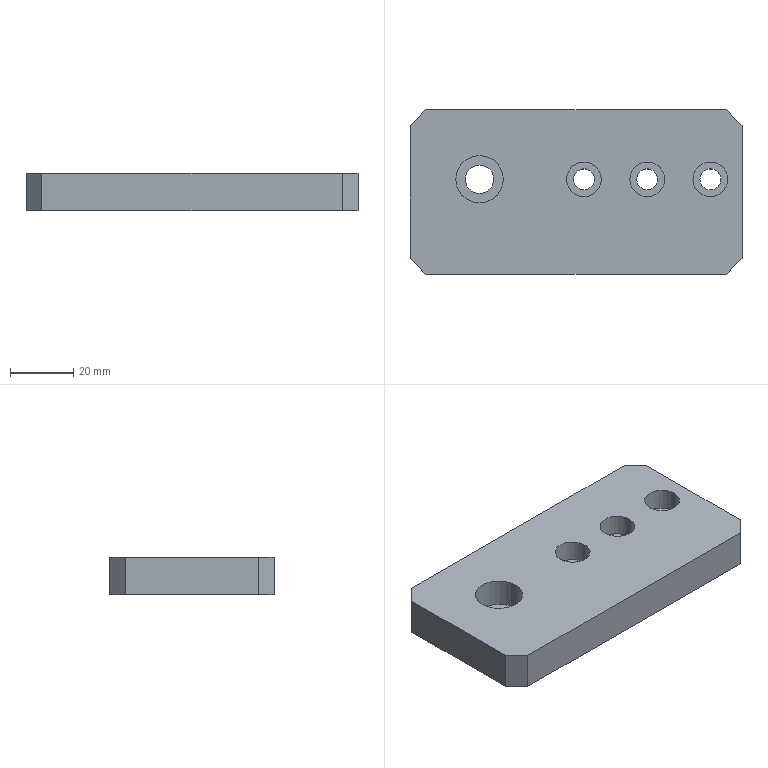Part | STEP file | Driven wheel fixing plate | 1 solid | 30 faces | box 105 x 52 x 12 mm | volume 60666 mm3 | cylinder 16 | plane 14 | commonest cylinder face diameters 6.6 x6 11 x6 9 x2 15 x2